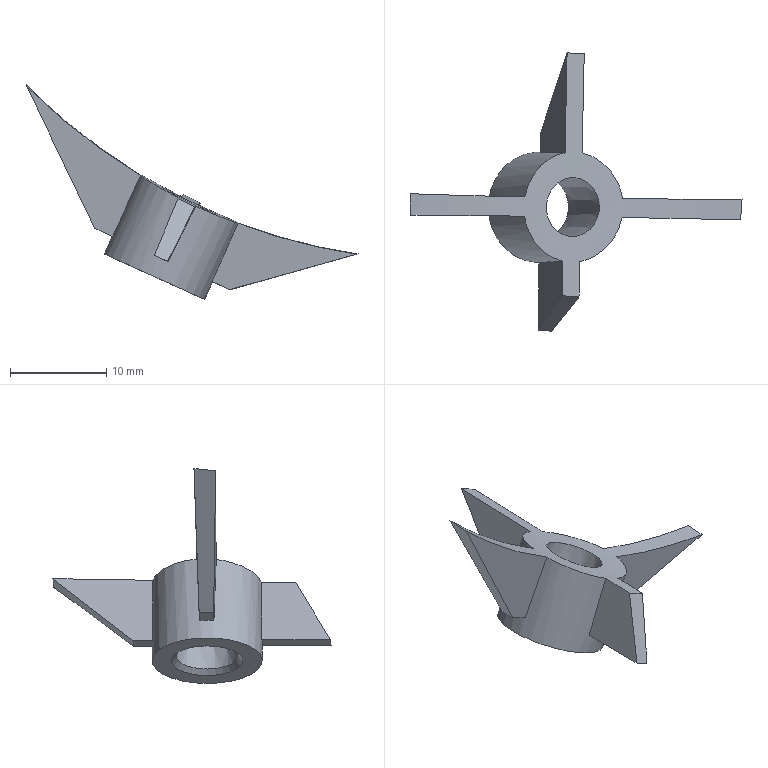Part | STEP file | solid 276 | 1 solid | 21 faces | box 34.494 x 28.911 x 22.331 mm | volume 948.282 mm3 | plane 16 | cone 2 | spline 2 | cylinder 1 | commonest cylinder face diameters 11.457 x1